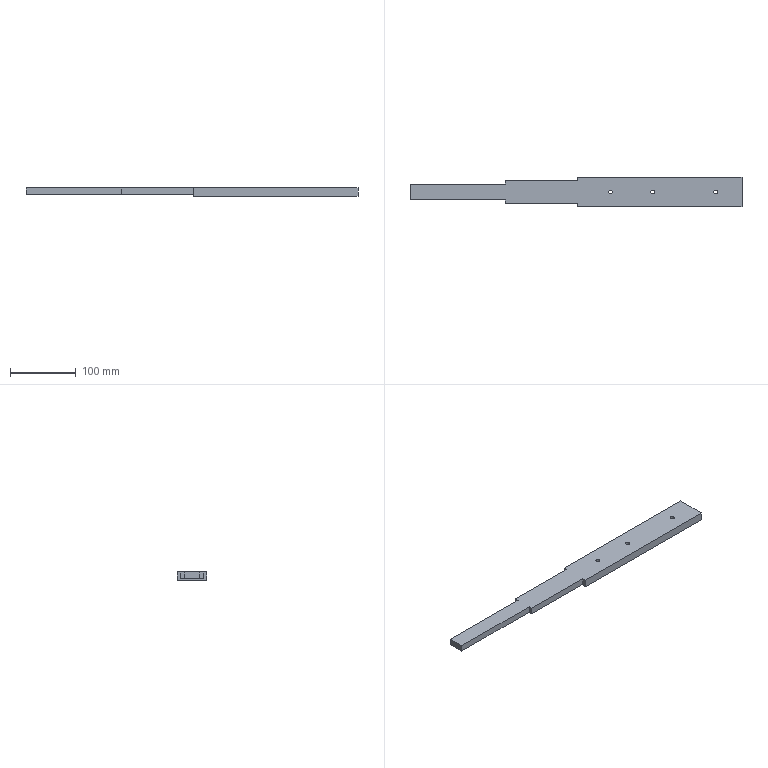Part | STEP file | Guide wheel mechanism revised.sldasm-Part-193 | 1 solid | 20 faces | box 505 x 45 x 12.5 mm | volume 214790 mm3 | plane 14 | cylinder 6 | commonest cylinder face diameters 6 x6
STEP:
#1=CARTESIAN_POINT('',(-78.,0.,12.5));
#2=VERTEX_POINT('',#1);
#3=CARTESIAN_POINT('',(-72.,0.,12.5));
#4=VERTEX_POINT('',#3);
#5=CARTESIAN_POINT('',(-75.,0.,12.5));
#6=DIRECTION('',(0.,0.,1.));
#7=DIRECTION('',(1.,0.,0.));
#8=AXIS2_PLACEMENT_3D('',#5,#6,#7);
#9=CIRCLE('',#8,3.);
#10=EDGE_CURVE('',#2,#4,#9,.T.);
#11=ORIENTED_EDGE('',*,*,#10,.T.);
#12=CARTESIAN_POINT('',(-72.,0.,0.));
#13=VERTEX_POINT('',#12);
#14=CARTESIAN_POINT('',(-72.,0.,12.5));
#15=DIRECTION('',(0.,0.,-1.));
#16=VECTOR('',#15,1000.);
#17=LINE('',#14,#16);
#18=EDGE_CURVE('',#4,#13,#17,.T.);
#19=ORIENTED_EDGE('',*,*,#18,.T.);
#20=CARTESIAN_POINT('',(-78.,0.,0.));
#21=VERTEX_POINT('',#20);
#22=CARTESIAN_POINT('',(-75.,0.,0.));
#23=DIRECTION('',(0.,0.,-1.));
#24=DIRECTION('',(-1.,0.,0.));
#25=AXIS2_PLACEMENT_3D('',#22,#23,#24);
#26=CIRCLE('',#25,3.);
#27=EDGE_CURVE('',#13,#21,#26,.T.);
#28=ORIENTED_EDGE('',*,*,#27,.T.);
#29=CARTESIAN_POINT('',(-78.,0.,12.5));
#30=DIRECTION('',(0.,0.,-1.));
#31=VECTOR('',#30,1000.);
#32=LINE('',#29,#31);
#33=EDGE_CURVE('',#2,#21,#32,.T.);
#34=ORIENTED_EDGE('',*,*,#33,.F.);
#35=EDGE_LOOP('',(#11,#19,#28,#34));
#36=FACE_OUTER_BOUND('',#35,.T.);
#37=CARTESIAN_POINT('',(-75.,0.,12.5));
#38=DIRECTION('',(0.,0.,-1.));
#39=DIRECTION('',(-1.,0.,0.));
#40=AXIS2_PLACEMENT_3D('',#37,#38,#39);
#41=CYLINDRICAL_SURFACE('',#40,3.);
#42=ADVANCED_FACE('',(#36),#41,.F.);
#43=CARTESIAN_POINT('',(-14.,0.,12.5));
#44=VERTEX_POINT('',#43);
#45=CARTESIAN_POINT('',(-8.,0.,12.5));
#46=VERTEX_POINT('',#45);
#47=CARTESIAN_POINT('',(-11.,0.,12.5));
#48=DIRECTION('',(0.,0.,1.));
#49=DIRECTION('',(1.,0.,0.));
#50=AXIS2_PLACEMENT_3D('',#47,#48,#49);
#51=CIRCLE('',#50,3.);
#52=EDGE_CURVE('',#44,#46,#51,.T.);
#53=ORIENTED_EDGE('',*,*,#52,.T.);
#54=CARTESIAN_POINT('',(-8.,0.,0.));
#55=VERTEX_POINT('',#54);
#56=CARTESIAN_POINT('',(-8.,0.,12.5));
#57=DIRECTION('',(0.,0.,-1.));
#58=VECTOR('',#57,1000.);
#59=LINE('',#56,#58);
#60=EDGE_CURVE('',#46,#55,#59,.T.);
#61=ORIENTED_EDGE('',*,*,#60,.T.);
#62=CARTESIAN_POINT('',(-14.,0.,0.));
#63=VERTEX_POINT('',#62);
#64=CARTESIAN_POINT('',(-11.,0.,0.));
#65=DIRECTION('',(0.,0.,-1.));
#66=DIRECTION('',(-1.,0.,0.));
#67=AXIS2_PLACEMENT_3D('',#64,#65,#66);
#68=CIRCLE('',#67,3.);
#69=EDGE_CURVE('',#55,#63,#68,.T.);
#70=ORIENTED_EDGE('',*,*,#69,.T.);
#71=CARTESIAN_POINT('',(-14.,0.,12.5));
#72=DIRECTION('',(0.,0.,-1.));
#73=VECTOR('',#72,1000.);
#74=LINE('',#71,#73);
#75=EDGE_CURVE('',#44,#63,#74,.T.);
#76=ORIENTED_EDGE('',*,*,#75,.F.);
#77=EDGE_LOOP('',(#53,#61,#70,#76));
#78=FACE_OUTER_BOUND('',#77,.T.);
#79=CARTESIAN_POINT('',(-11.,0.,12.5));
#80=DIRECTION('',(0.,0.,-1.));
#81=DIRECTION('',(-1.,0.,0.));
#82=AXIS2_PLACEMENT_3D('',#79,#80,#81);
#83=CYLINDRICAL_SURFACE('',#82,3.);
#84=ADVANCED_FACE('',(#78),#83,.F.);
#85=CARTESIAN_POINT('',(82.,0.,12.5));
#86=VERTEX_POINT('',#85);
#87=CARTESIAN_POINT('',(88.,0.,12.5));
#88=VERTEX_POINT('',#87);
#89=CARTESIAN_POINT('',(85.,0.,12.5));
#90=DIRECTION('',(0.,0.,1.));
#91=DIRECTION('',(1.,0.,0.));
#92=AXIS2_PLACEMENT_3D('',#89,#90,#91);
#93=CIRCLE('',#92,3.);
#94=EDGE_CURVE('',#86,#88,#93,.T.);
#95=ORIENTED_EDGE('',*,*,#94,.T.);
#96=CARTESIAN_POINT('',(88.,0.,0.));
#97=VERTEX_POINT('',#96);
#98=CARTESIAN_POINT('',(88.,0.,12.5));
#99=DIRECTION('',(0.,0.,-1.));
#100=VECTOR('',#99,1000.);
#101=LINE('',#98,#100);
#102=EDGE_CURVE('',#88,#97,#101,.T.);
#103=ORIENTED_EDGE('',*,*,#102,.T.);
#104=CARTESIAN_POINT('',(82.,0.,0.));
#105=VERTEX_POINT('',#104);
#106=CARTESIAN_POINT('',(85.,0.,0.));
#107=DIRECTION('',(0.,0.,-1.));
#108=DIRECTION('',(-1.,0.,0.));
#109=AXIS2_PLACEMENT_3D('',#106,#107,#108);
#110=CIRCLE('',#109,3.);
#111=EDGE_CURVE('',#97,#105,#110,.T.);
#112=ORIENTED_EDGE('',*,*,#111,.T.);
#113=CARTESIAN_POINT('',(82.,0.,12.5));
#114=DIRECTION('',(0.,0.,-1.));
#115=VECTOR('',#114,1000.);
#116=LINE('',#113,#115);
#117=EDGE_CURVE('',#86,#105,#116,.T.);
#118=ORIENTED_EDGE('',*,*,#117,.F.);
#119=EDGE_LOOP('',(#95,#103,#112,#118));
#120=FACE_OUTER_BOUND('',#119,.T.);
#121=CARTESIAN_POINT('',(85.,0.,12.5));
#122=DIRECTION('',(0.,0.,-1.));
#123=DIRECTION('',(-1.,0.,0.));
#124=AXIS2_PLACEMENT_3D('',#121,#122,#123);
#125=CYLINDRICAL_SURFACE('',#124,3.);
#126=ADVANCED_FACE('',(#120),#125,.F.);
#127=CARTESIAN_POINT('',(-125.,-17.5,2.));
#128=VERTEX_POINT('',#127);
#129=CARTESIAN_POINT('',(-125.,-17.5,12.5));
#130=VERTEX_POINT('',#129);
#131=CARTESIAN_POINT('',(-125.,-17.5,2.));
#132=DIRECTION('',(0.,0.,1.));
#133=VECTOR('',#132,1000.);
#134=LINE('',#131,#133);
#135=EDGE_CURVE('',#128,#130,#134,.T.);
#136=ORIENTED_EDGE('',*,*,#135,.F.);
#137=CARTESIAN_POINT('',(-125.,17.5,2.));
#138=VERTEX_POINT('',#137);
#139=CARTESIAN_POINT('',(-125.,17.5,2.));
#140=DIRECTION('',(0.,1.,0.));
#141=VECTOR('',#140,1000.);
#142=LINE('',#139,#141);
#143=EDGE_CURVE('',#128,#138,#142,.T.);
#144=ORIENTED_EDGE('',*,*,#143,.T.);
#145=CARTESIAN_POINT('',(-125.,17.5,12.5));
#146=VERTEX_POINT('',#145);
#147=CARTESIAN_POINT('',(-125.,17.5,2.));
#148=DIRECTION('',(0.,0.,1.));
#149=VECTOR('',#148,1000.);
#150=LINE('',#147,#149);
#151=EDGE_CURVE('',#138,#146,#150,.T.);
#152=ORIENTED_EDGE('',*,*,#151,.T.);
#153=CARTESIAN_POINT('',(-125.,22.5,12.5));
#154=VERTEX_POINT('',#153);
#155=CARTESIAN_POINT('',(-125.,22.5,12.5));
#156=DIRECTION('',(0.,-1.,0.));
#157=VECTOR('',#156,1000.);
#158=LINE('',#155,#157);
#159=EDGE_CURVE('',#154,#146,#158,.T.);
#160=ORIENTED_EDGE('',*,*,#159,.F.);
#161=CARTESIAN_POINT('',(-125.,22.5,0.));
#162=VERTEX_POINT('',#161);
#163=CARTESIAN_POINT('',(-125.,22.5,12.5));
#164=DIRECTION('',(0.,0.,-1.));
#165=VECTOR('',#164,1000.);
#166=LINE('',#163,#165);
#167=EDGE_CURVE('',#154,#162,#166,.T.);
#168=ORIENTED_EDGE('',*,*,#167,.T.);
#169=CARTESIAN_POINT('',(-125.,-22.5,0.));
#170=VERTEX_POINT('',#169);
#171=CARTESIAN_POINT('',(-125.,22.5,0.));
#172=DIRECTION('',(0.,-1.,0.));
#173=VECTOR('',#172,1000.);
#174=LINE('',#171,#173);
#175=EDGE_CURVE('',#162,#170,#174,.T.);
#176=ORIENTED_EDGE('',*,*,#175,.T.);
#177=CARTESIAN_POINT('',(-125.,-22.5,12.5));
#178=VERTEX_POINT('',#177);
#179=CARTESIAN_POINT('',(-125.,-22.5,12.5));
#180=DIRECTION('',(0.,0.,-1.));
#181=VECTOR('',#180,1000.);
#182=LINE('',#179,#181);
#183=EDGE_CURVE('',#178,#170,#182,.T.);
#184=ORIENTED_EDGE('',*,*,#183,.F.);
#185=CARTESIAN_POINT('',(-125.,22.5,12.5));
#186=DIRECTION('',(0.,-1.,0.));
#187=VECTOR('',#186,1000.);
#188=LINE('',#185,#187);
#189=EDGE_CURVE('',#130,#178,#188,.T.);
#190=ORIENTED_EDGE('',*,*,#189,.F.);
#191=EDGE_LOOP('',(#136,#144,#152,#160,#168,#176,#184,#190));
#192=FACE_OUTER_BOUND('',#191,.T.);
#193=CARTESIAN_POINT('',(-125.,22.5,12.5));
#194=DIRECTION('',(1.,0.,0.));
#195=DIRECTION('',(0.,0.,-1.));
#196=AXIS2_PLACEMENT_3D('',#193,#194,#195);
#197=PLANE('',#196);
#198=ADVANCED_FACE('',(#192),#197,.F.);
#199=CARTESIAN_POINT('',(125.,-22.5,0.));
#200=VERTEX_POINT('',#199);
#201=CARTESIAN_POINT('',(125.,22.5,0.));
#202=VERTEX_POINT('',#201);
#203=CARTESIAN_POINT('',(125.,22.5,0.));
#204=DIRECTION('',(0.,1.,0.));
#205=VECTOR('',#204,1000.);
#206=LINE('',#203,#205);
#207=EDGE_CURVE('',#200,#202,#206,.T.);
#208=ORIENTED_EDGE('',*,*,#207,.T.);
#209=CARTESIAN_POINT('',(125.,22.5,12.5));
#210=VERTEX_POINT('',#209);
#211=CARTESIAN_POINT('',(125.,22.5,12.5));
#212=DIRECTION('',(0.,0.,-1.));
#213=VECTOR('',#212,1000.);
#214=LINE('',#211,#213);
#215=EDGE_CURVE('',#210,#202,#214,.T.);
#216=ORIENTED_EDGE('',*,*,#215,.F.);
#217=CARTESIAN_POINT('',(125.,-22.5,12.5));
#218=VERTEX_POINT('',#217);
#219=CARTESIAN_POINT('',(125.,22.5,12.5));
#220=DIRECTION('',(0.,1.,0.));
#221=VECTOR('',#220,1000.);
#222=LINE('',#219,#221);
#223=EDGE_CURVE('',#218,#210,#222,.T.);
#224=ORIENTED_EDGE('',*,*,#223,.F.);
#225=CARTESIAN_POINT('',(125.,-22.5,12.5));
#226=DIRECTION('',(0.,0.,-1.));
#227=VECTOR('',#226,1000.);
#228=LINE('',#225,#227);
#229=EDGE_CURVE('',#218,#200,#228,.T.);
#230=ORIENTED_EDGE('',*,*,#229,.T.);
#231=EDGE_LOOP('',(#208,#216,#224,#230));
#232=FACE_OUTER_BOUND('',#231,.T.);
#233=CARTESIAN_POINT('',(125.,22.5,12.5));
#234=DIRECTION('',(-1.,0.,0.));
#235=DIRECTION('',(0.,0.,1.));
#236=AXIS2_PLACEMENT_3D('',#233,#234,#235);
#237=PLANE('',#236);
#238=ADVANCED_FACE('',(#232),#237,.F.);
#239=CARTESIAN_POINT('',(-125.,22.5,0.));
#240=DIRECTION('',(-1.,0.,0.));
#241=VECTOR('',#240,1000.);
#242=LINE('',#239,#241);
#243=EDGE_CURVE('',#202,#162,#242,.T.);
#244=ORIENTED_EDGE('',*,*,#243,.T.);
#245=ORIENTED_EDGE('',*,*,#167,.F.);
#246=CARTESIAN_POINT('',(-125.,22.5,12.5));
#247=DIRECTION('',(-1.,0.,0.));
#248=VECTOR('',#247,1000.);
#249=LINE('',#246,#248);
#250=EDGE_CURVE('',#210,#154,#249,.T.);
#251=ORIENTED_EDGE('',*,*,#250,.F.);
#252=ORIENTED_EDGE('',*,*,#215,.T.);
#253=EDGE_LOOP('',(#244,#245,#251,#252));
#254=FACE_OUTER_BOUND('',#253,.T.);
#255=CARTESIAN_POINT('',(-125.,22.5,12.5));
#256=DIRECTION('',(0.,-1.,0.));
#257=DIRECTION('',(0.,0.,-1.));
#258=AXIS2_PLACEMENT_3D('',#255,#256,#257);
#259=PLANE('',#258);
#260=ADVANCED_FACE('',(#254),#259,.F.);
#261=CARTESIAN_POINT('',(-125.,-22.5,0.));
#262=DIRECTION('',(1.,0.,0.));
#263=VECTOR('',#262,1000.);
#264=LINE('',#261,#263);
#265=EDGE_CURVE('',#170,#200,#264,.T.);
#266=ORIENTED_EDGE('',*,*,#265,.T.);
#267=ORIENTED_EDGE('',*,*,#229,.F.);
#268=CARTESIAN_POINT('',(-125.,-22.5,12.5));
#269=DIRECTION('',(1.,0.,0.));
#270=VECTOR('',#269,1000.);
#271=LINE('',#268,#270);
#272=EDGE_CURVE('',#178,#218,#271,.T.);
#273=ORIENTED_EDGE('',*,*,#272,.F.);
#274=ORIENTED_EDGE('',*,*,#183,.T.);
#275=EDGE_LOOP('',(#266,#267,#273,#274));
#276=FACE_OUTER_BOUND('',#275,.T.);
#277=CARTESIAN_POINT('',(-125.,-22.5,12.5));
#278=DIRECTION('',(0.,1.,0.));
#279=DIRECTION('',(0.,0.,1.));
#280=AXIS2_PLACEMENT_3D('',#277,#278,#279);
#281=PLANE('',#280);
#282=ADVANCED_FACE('',(#276),#281,.F.);
#283=ORIENTED_EDGE('',*,*,#10,.F.);
#284=CARTESIAN_POINT('',(-75.,0.,12.5));
#285=DIRECTION('',(0.,0.,1.));
#286=DIRECTION('',(1.,0.,0.));
#287=AXIS2_PLACEMENT_3D('',#284,#285,#286);
#288=CIRCLE('',#287,3.);
#289=EDGE_CURVE('',#4,#2,#288,.T.);
#290=ORIENTED_EDGE('',*,*,#289,.F.);
#291=EDGE_LOOP('',(#283,#290));
#292=FACE_BOUND('',#291,.T.);
#293=ORIENTED_EDGE('',*,*,#52,.F.);
#294=CARTESIAN_POINT('',(-11.,0.,12.5));
#295=DIRECTION('',(0.,0.,1.));
#296=DIRECTION('',(1.,0.,0.));
#297=AXIS2_PLACEMENT_3D('',#294,#295,#296);
#298=CIRCLE('',#297,3.);
#299=EDGE_CURVE('',#46,#44,#298,.T.);
#300=ORIENTED_EDGE('',*,*,#299,.F.);
#301=EDGE_LOOP('',(#293,#300));
#302=FACE_BOUND('',#301,.T.);
#303=ORIENTED_EDGE('',*,*,#94,.F.);
#304=CARTESIAN_POINT('',(85.,0.,12.5));
#305=DIRECTION('',(0.,0.,1.));
#306=DIRECTION('',(1.,0.,0.));
#307=AXIS2_PLACEMENT_3D('',#304,#305,#306);
#308=CIRCLE('',#307,3.);
#309=EDGE_CURVE('',#88,#86,#308,.T.);
#310=ORIENTED_EDGE('',*,*,#309,.F.);
#311=EDGE_LOOP('',(#303,#310));
#312=FACE_BOUND('',#311,.T.);
#313=ORIENTED_EDGE('',*,*,#223,.T.);
#314=ORIENTED_EDGE('',*,*,#250,.T.);
#315=ORIENTED_EDGE('',*,*,#159,.T.);
#316=CARTESIAN_POINT('',(-235.,17.5,12.5));
#317=VERTEX_POINT('',#316);
#318=CARTESIAN_POINT('',(-125.,17.5,12.5));
#319=DIRECTION('',(-1.,0.,0.));
#320=VECTOR('',#319,1000.);
#321=LINE('',#318,#320);
#322=EDGE_CURVE('',#146,#317,#321,.T.);
#323=ORIENTED_EDGE('',*,*,#322,.T.);
#324=CARTESIAN_POINT('',(-235.,12.,12.5));
#325=VERTEX_POINT('',#324);
#326=CARTESIAN_POINT('',(-235.,17.5,12.5));
#327=DIRECTION('',(0.,-1.,0.));
#328=VECTOR('',#327,1000.);
#329=LINE('',#326,#328);
#330=EDGE_CURVE('',#317,#325,#329,.T.);
#331=ORIENTED_EDGE('',*,*,#330,.T.);
#332=CARTESIAN_POINT('',(-380.,12.,12.5));
#333=VERTEX_POINT('',#332);
#334=CARTESIAN_POINT('',(-235.,12.,12.5));
#335=DIRECTION('',(-1.,0.,0.));
#336=VECTOR('',#335,1000.);
#337=LINE('',#334,#336);
#338=EDGE_CURVE('',#325,#333,#337,.T.);
#339=ORIENTED_EDGE('',*,*,#338,.T.);
#340=CARTESIAN_POINT('',(-380.,-12.,12.5));
#341=VERTEX_POINT('',#340);
#342=CARTESIAN_POINT('',(-380.,-12.,12.5));
#343=DIRECTION('',(0.,-1.,0.));
#344=VECTOR('',#343,1000.);
#345=LINE('',#342,#344);
#346=EDGE_CURVE('',#333,#341,#345,.T.);
#347=ORIENTED_EDGE('',*,*,#346,.T.);
#348=CARTESIAN_POINT('',(-235.,-12.,12.5));
#349=VERTEX_POINT('',#348);
#350=CARTESIAN_POINT('',(-235.,-12.,12.5));
#351=DIRECTION('',(1.,0.,0.));
#352=VECTOR('',#351,1000.);
#353=LINE('',#350,#352);
#354=EDGE_CURVE('',#341,#349,#353,.T.);
#355=ORIENTED_EDGE('',*,*,#354,.T.);
#356=CARTESIAN_POINT('',(-235.,-17.5,12.5));
#357=VERTEX_POINT('',#356);
#358=CARTESIAN_POINT('',(-235.,17.5,12.5));
#359=DIRECTION('',(0.,-1.,0.));
#360=VECTOR('',#359,1000.);
#361=LINE('',#358,#360);
#362=EDGE_CURVE('',#349,#357,#361,.T.);
#363=ORIENTED_EDGE('',*,*,#362,.T.);
#364=CARTESIAN_POINT('',(-125.,-17.5,12.5));
#365=DIRECTION('',(1.,0.,0.));
#366=VECTOR('',#365,1000.);
#367=LINE('',#364,#366);
#368=EDGE_CURVE('',#357,#130,#367,.T.);
#369=ORIENTED_EDGE('',*,*,#368,.T.);
#370=ORIENTED_EDGE('',*,*,#189,.T.);
#371=ORIENTED_EDGE('',*,*,#272,.T.);
#372=EDGE_LOOP('',(#313,#314,#315,#323,#331,#339,#347,#355,#363,#369,#370,#371));
#373=FACE_OUTER_BOUND('',#372,.T.);
#374=CARTESIAN_POINT('',(125.,-22.5,12.5));
#375=DIRECTION('',(0.,0.,1.));
#376=DIRECTION('',(1.,0.,0.));
#377=AXIS2_PLACEMENT_3D('',#374,#375,#376);
#378=PLANE('',#377);
#379=ADVANCED_FACE('',(#292,#302,#312,#373),#378,.T.);
#380=CARTESIAN_POINT('',(-75.,0.,0.));
#381=DIRECTION('',(0.,0.,-1.));
#382=DIRECTION('',(-1.,0.,0.));
#383=AXIS2_PLACEMENT_3D('',#380,#381,#382);
#384=CIRCLE('',#383,3.);
#385=EDGE_CURVE('',#21,#13,#384,.T.);
#386=ORIENTED_EDGE('',*,*,#385,.F.);
#387=ORIENTED_EDGE('',*,*,#27,.F.);
#388=EDGE_LOOP('',(#386,#387));
#389=FACE_BOUND('',#388,.T.);
#390=CARTESIAN_POINT('',(-11.,0.,0.));
#391=DIRECTION('',(0.,0.,-1.));
#392=DIRECTION('',(-1.,0.,0.));
#393=AXIS2_PLACEMENT_3D('',#390,#391,#392);
#394=CIRCLE('',#393,3.);
#395=EDGE_CURVE('',#63,#55,#394,.T.);
#396=ORIENTED_EDGE('',*,*,#395,.F.);
#397=ORIENTED_EDGE('',*,*,#69,.F.);
#398=EDGE_LOOP('',(#396,#397));
#399=FACE_BOUND('',#398,.T.);
#400=CARTESIAN_POINT('',(85.,0.,0.));
#401=DIRECTION('',(0.,0.,-1.));
#402=DIRECTION('',(-1.,0.,0.));
#403=AXIS2_PLACEMENT_3D('',#400,#401,#402);
#404=CIRCLE('',#403,3.);
#405=EDGE_CURVE('',#105,#97,#404,.T.);
#406=ORIENTED_EDGE('',*,*,#405,.F.);
#407=ORIENTED_EDGE('',*,*,#111,.F.);
#408=EDGE_LOOP('',(#406,#407));
#409=FACE_BOUND('',#408,.T.);
#410=ORIENTED_EDGE('',*,*,#207,.F.);
#411=ORIENTED_EDGE('',*,*,#265,.F.);
#412=ORIENTED_EDGE('',*,*,#175,.F.);
#413=ORIENTED_EDGE('',*,*,#243,.F.);
#414=EDGE_LOOP('',(#410,#411,#412,#413));
#415=FACE_OUTER_BOUND('',#414,.T.);
#416=CARTESIAN_POINT('',(125.,-22.5,0.));
#417=DIRECTION('',(0.,0.,1.));
#418=DIRECTION('',(1.,0.,0.));
#419=AXIS2_PLACEMENT_3D('',#416,#417,#418);
#420=PLANE('',#419);
#421=ADVANCED_FACE('',(#389,#399,#409,#415),#420,.F.);
#422=ORIENTED_EDGE('',*,*,#368,.F.);
#423=CARTESIAN_POINT('',(-235.,-17.5,2.));
#424=VERTEX_POINT('',#423);
#425=CARTESIAN_POINT('',(-235.,-17.5,2.));
#426=DIRECTION('',(0.,0.,1.));
#427=VECTOR('',#426,1000.);
#428=LINE('',#425,#427);
#429=EDGE_CURVE('',#424,#357,#428,.T.);
#430=ORIENTED_EDGE('',*,*,#429,.F.);
#431=CARTESIAN_POINT('',(-125.,-17.5,2.));
#432=DIRECTION('',(1.,0.,0.));
#433=VECTOR('',#432,1000.);
#434=LINE('',#431,#433);
#435=EDGE_CURVE('',#424,#128,#434,.T.);
#436=ORIENTED_EDGE('',*,*,#435,.T.);
#437=ORIENTED_EDGE('',*,*,#135,.T.);
#438=EDGE_LOOP('',(#422,#430,#436,#437));
#439=FACE_OUTER_BOUND('',#438,.T.);
#440=CARTESIAN_POINT('',(-125.,-17.5,2.));
#441=DIRECTION('',(0.,-1.,0.));
#442=DIRECTION('',(1.,0.,0.));
#443=AXIS2_PLACEMENT_3D('',#440,#441,#442);
#444=PLANE('',#443);
#445=ADVANCED_FACE('',(#439),#444,.T.);
#446=CARTESIAN_POINT('',(-235.,-12.,2.5));
#447=VERTEX_POINT('',#446);
#448=CARTESIAN_POINT('',(-235.,-12.,2.5));
#449=DIRECTION('',(0.,0.,1.));
#450=VECTOR('',#449,1000.);
#451=LINE('',#448,#450);
#452=EDGE_CURVE('',#447,#349,#451,.T.);
#453=ORIENTED_EDGE('',*,*,#452,.F.);
#454=CARTESIAN_POINT('',(-235.,12.,2.5));
#455=VERTEX_POINT('',#454);
#456=CARTESIAN_POINT('',(-235.,-12.,2.5));
#457=DIRECTION('',(0.,1.,0.));
#458=VECTOR('',#457,1000.);
#459=LINE('',#456,#458);
#460=EDGE_CURVE('',#447,#455,#459,.T.);
#461=ORIENTED_EDGE('',*,*,#460,.T.);
#462=CARTESIAN_POINT('',(-235.,12.,2.5));
#463=DIRECTION('',(0.,0.,1.));
#464=VECTOR('',#463,1000.);
#465=LINE('',#462,#464);
#466=EDGE_CURVE('',#455,#325,#465,.T.);
#467=ORIENTED_EDGE('',*,*,#466,.T.);
#468=ORIENTED_EDGE('',*,*,#330,.F.);
#469=CARTESIAN_POINT('',(-235.,17.5,2.));
#470=VERTEX_POINT('',#469);
#471=CARTESIAN_POINT('',(-235.,17.5,2.));
#472=DIRECTION('',(0.,0.,1.));
#473=VECTOR('',#472,1000.);
#474=LINE('',#471,#473);
#475=EDGE_CURVE('',#470,#317,#474,.T.);
#476=ORIENTED_EDGE('',*,*,#475,.F.);
#477=CARTESIAN_POINT('',(-235.,17.5,2.));
#478=DIRECTION('',(0.,-1.,0.));
#479=VECTOR('',#478,1000.);
#480=LINE('',#477,#479);
#481=EDGE_CURVE('',#470,#424,#480,.T.);
#482=ORIENTED_EDGE('',*,*,#481,.T.);
#483=ORIENTED_EDGE('',*,*,#429,.T.);
#484=ORIENTED_EDGE('',*,*,#362,.F.);
#485=EDGE_LOOP('',(#453,#461,#467,#468,#476,#482,#483,#484));
#486=FACE_OUTER_BOUND('',#485,.T.);
#487=CARTESIAN_POINT('',(-235.,17.5,2.));
#488=DIRECTION('',(-1.,0.,0.));
#489=DIRECTION('',(0.,0.,1.));
#490=AXIS2_PLACEMENT_3D('',#487,#488,#489);
#491=PLANE('',#490);
#492=ADVANCED_FACE('',(#486),#491,.T.);
#493=ORIENTED_EDGE('',*,*,#322,.F.);
#494=ORIENTED_EDGE('',*,*,#151,.F.);
#495=CARTESIAN_POINT('',(-125.,17.5,2.));
#496=DIRECTION('',(-1.,0.,0.));
#497=VECTOR('',#496,1000.);
#498=LINE('',#495,#497);
#499=EDGE_CURVE('',#138,#470,#498,.T.);
#500=ORIENTED_EDGE('',*,*,#499,.T.);
#501=ORIENTED_EDGE('',*,*,#475,.T.);
#502=EDGE_LOOP('',(#493,#494,#500,#501));
#503=FACE_OUTER_BOUND('',#502,.T.);
#504=CARTESIAN_POINT('',(-125.,17.5,2.));
#505=DIRECTION('',(0.,1.,0.));
#506=DIRECTION('',(-1.,0.,0.));
#507=AXIS2_PLACEMENT_3D('',#504,#505,#506);
#508=PLANE('',#507);
#509=ADVANCED_FACE('',(#503),#508,.T.);
#510=ORIENTED_EDGE('',*,*,#143,.F.);
#511=ORIENTED_EDGE('',*,*,#435,.F.);
#512=ORIENTED_EDGE('',*,*,#481,.F.);
#513=ORIENTED_EDGE('',*,*,#499,.F.);
#514=EDGE_LOOP('',(#510,#511,#512,#513));
#515=FACE_OUTER_BOUND('',#514,.T.);
#516=CARTESIAN_POINT('',(-125.,-17.5,2.));
#517=DIRECTION('',(0.,0.,-1.));
#518=DIRECTION('',(-1.,0.,0.));
#519=AXIS2_PLACEMENT_3D('',#516,#517,#518);
#520=PLANE('',#519);
#521=ADVANCED_FACE('',(#515),#520,.T.);
#522=ORIENTED_EDGE('',*,*,#102,.F.);
#523=ORIENTED_EDGE('',*,*,#309,.T.);
#524=ORIENTED_EDGE('',*,*,#117,.T.);
#525=ORIENTED_EDGE('',*,*,#405,.T.);
#526=EDGE_LOOP('',(#522,#523,#524,#525));
#527=FACE_OUTER_BOUND('',#526,.T.);
#528=CARTESIAN_POINT('',(85.,0.,12.5));
#529=DIRECTION('',(0.,0.,-1.));
#530=DIRECTION('',(-1.,0.,0.));
#531=AXIS2_PLACEMENT_3D('',#528,#529,#530);
#532=CYLINDRICAL_SURFACE('',#531,3.);
#533=ADVANCED_FACE('',(#527),#532,.F.);
#534=ORIENTED_EDGE('',*,*,#60,.F.);
#535=ORIENTED_EDGE('',*,*,#299,.T.);
#536=ORIENTED_EDGE('',*,*,#75,.T.);
#537=ORIENTED_EDGE('',*,*,#395,.T.);
#538=EDGE_LOOP('',(#534,#535,#536,#537));
#539=FACE_OUTER_BOUND('',#538,.T.);
#540=CARTESIAN_POINT('',(-11.,0.,12.5));
#541=DIRECTION('',(0.,0.,-1.));
#542=DIRECTION('',(-1.,0.,0.));
#543=AXIS2_PLACEMENT_3D('',#540,#541,#542);
#544=CYLINDRICAL_SURFACE('',#543,3.);
#545=ADVANCED_FACE('',(#539),#544,.F.);
#546=ORIENTED_EDGE('',*,*,#18,.F.);
#547=ORIENTED_EDGE('',*,*,#289,.T.);
#548=ORIENTED_EDGE('',*,*,#33,.T.);
#549=ORIENTED_EDGE('',*,*,#385,.T.);
#550=EDGE_LOOP('',(#546,#547,#548,#549));
#551=FACE_OUTER_BOUND('',#550,.T.);
#552=CARTESIAN_POINT('',(-75.,0.,12.5));
#553=DIRECTION('',(0.,0.,-1.));
#554=DIRECTION('',(-1.,0.,0.));
#555=AXIS2_PLACEMENT_3D('',#552,#553,#554);
#556=CYLINDRICAL_SURFACE('',#555,3.);
#557=ADVANCED_FACE('',(#551),#556,.F.);
#558=ORIENTED_EDGE('',*,*,#354,.F.);
#559=CARTESIAN_POINT('',(-380.,-12.,2.5));
#560=VERTEX_POINT('',#559);
#561=CARTESIAN_POINT('',(-380.,-12.,2.5));
#562=DIRECTION('',(0.,0.,1.));
#563=VECTOR('',#562,1000.);
#564=LINE('',#561,#563);
#565=EDGE_CURVE('',#560,#341,#564,.T.);
#566=ORIENTED_EDGE('',*,*,#565,.F.);
#567=CARTESIAN_POINT('',(-235.,-12.,2.5));
#568=DIRECTION('',(1.,0.,0.));
#569=VECTOR('',#568,1000.);
#570=LINE('',#567,#569);
#571=EDGE_CURVE('',#560,#447,#570,.T.);
#572=ORIENTED_EDGE('',*,*,#571,.T.);
#573=ORIENTED_EDGE('',*,*,#452,.T.);
#574=EDGE_LOOP('',(#558,#566,#572,#573));
#575=FACE_OUTER_BOUND('',#574,.T.);
#576=CARTESIAN_POINT('',(-235.,-12.,2.5));
#577=DIRECTION('',(0.,-1.,0.));
#578=DIRECTION('',(1.,0.,0.));
#579=AXIS2_PLACEMENT_3D('',#576,#577,#578);
#580=PLANE('',#579);
#581=ADVANCED_FACE('',(#575),#580,.T.);
#582=ORIENTED_EDGE('',*,*,#346,.F.);
#583=CARTESIAN_POINT('',(-380.,12.,2.5));
#584=VERTEX_POINT('',#583);
#585=CARTESIAN_POINT('',(-380.,12.,2.5));
#586=DIRECTION('',(0.,0.,1.));
#587=VECTOR('',#586,1000.);
#588=LINE('',#585,#587);
#589=EDGE_CURVE('',#584,#333,#588,.T.);
#590=ORIENTED_EDGE('',*,*,#589,.F.);
#591=CARTESIAN_POINT('',(-380.,-12.,2.5));
#592=DIRECTION('',(0.,-1.,0.));
#593=VECTOR('',#592,1000.);
#594=LINE('',#591,#593);
#595=EDGE_CURVE('',#584,#560,#594,.T.);
#596=ORIENTED_EDGE('',*,*,#595,.T.);
#597=ORIENTED_EDGE('',*,*,#565,.T.);
#598=EDGE_LOOP('',(#582,#590,#596,#597));
#599=FACE_OUTER_BOUND('',#598,.T.);
#600=CARTESIAN_POINT('',(-380.,-12.,2.5));
#601=DIRECTION('',(-1.,0.,0.));
#602=DIRECTION('',(0.,0.,1.));
#603=AXIS2_PLACEMENT_3D('',#600,#601,#602);
#604=PLANE('',#603);
#605=ADVANCED_FACE('',(#599),#604,.T.);
#606=ORIENTED_EDGE('',*,*,#338,.F.);
#607=ORIENTED_EDGE('',*,*,#466,.F.);
#608=CARTESIAN_POINT('',(-235.,12.,2.5));
#609=DIRECTION('',(-1.,0.,0.));
#610=VECTOR('',#609,1000.);
#611=LINE('',#608,#610);
#612=EDGE_CURVE('',#455,#584,#611,.T.);
#613=ORIENTED_EDGE('',*,*,#612,.T.);
#614=ORIENTED_EDGE('',*,*,#589,.T.);
#615=EDGE_LOOP('',(#606,#607,#613,#614));
#616=FACE_OUTER_BOUND('',#615,.T.);
#617=CARTESIAN_POINT('',(-235.,12.,2.5));
#618=DIRECTION('',(0.,1.,0.));
#619=DIRECTION('',(-1.,0.,0.));
#620=AXIS2_PLACEMENT_3D('',#617,#618,#619);
#621=PLANE('',#620);
#622=ADVANCED_FACE('',(#616),#621,.T.);
#623=ORIENTED_EDGE('',*,*,#460,.F.);
#624=ORIENTED_EDGE('',*,*,#571,.F.);
#625=ORIENTED_EDGE('',*,*,#595,.F.);
#626=ORIENTED_EDGE('',*,*,#612,.F.);
#627=EDGE_LOOP('',(#623,#624,#625,#626));
#628=FACE_OUTER_BOUND('',#627,.T.);
#629=CARTESIAN_POINT('',(-235.,12.,2.5));
#630=DIRECTION('',(0.,0.,1.));
#631=DIRECTION('',(1.,0.,0.));
#632=AXIS2_PLACEMENT_3D('',#629,#630,#631);
#633=PLANE('',#632);
#634=ADVANCED_FACE('',(#628),#633,.F.);
#635=CLOSED_SHELL('',(#42,#84,#126,#198,#238,#260,#282,#379,#421,#445,#492,#509,#521,#533,#545,#557,#581,#605,#622,#634));
#636=MANIFOLD_SOLID_BREP('',#635);
#637=CARTESIAN_POINT('',(0.,0.,0.));
#638=DIRECTION('',(0.,0.,1.));
#639=DIRECTION('',(1.,0.,0.));
#640=AXIS2_PLACEMENT_3D('',#637,#638,#639);
#641=(LENGTH_UNIT()NAMED_UNIT(*)SI_UNIT(.MILLI.,.METRE.));
#642=UNCERTAINTY_MEASURE_WITH_UNIT(LENGTH_MEASURE(0.00001),#641,'','');
#643=(NAMED_UNIT(*)PLANE_ANGLE_UNIT()SI_UNIT($,.RADIAN.));
#644=(NAMED_UNIT(*)SI_UNIT($,.STERADIAN.)SOLID_ANGLE_UNIT());
#645=(GEOMETRIC_REPRESENTATION_CONTEXT(3)GLOBAL_UNCERTAINTY_ASSIGNED_CONTEXT((#642))GLOBAL_UNIT_ASSIGNED_CONTEXT((#641,#643,#644))REPRESENTATION_CONTEXT('',''));
#646=ADVANCED_BREP_SHAPE_REPRESENTATION('',(#636,#640),#645);